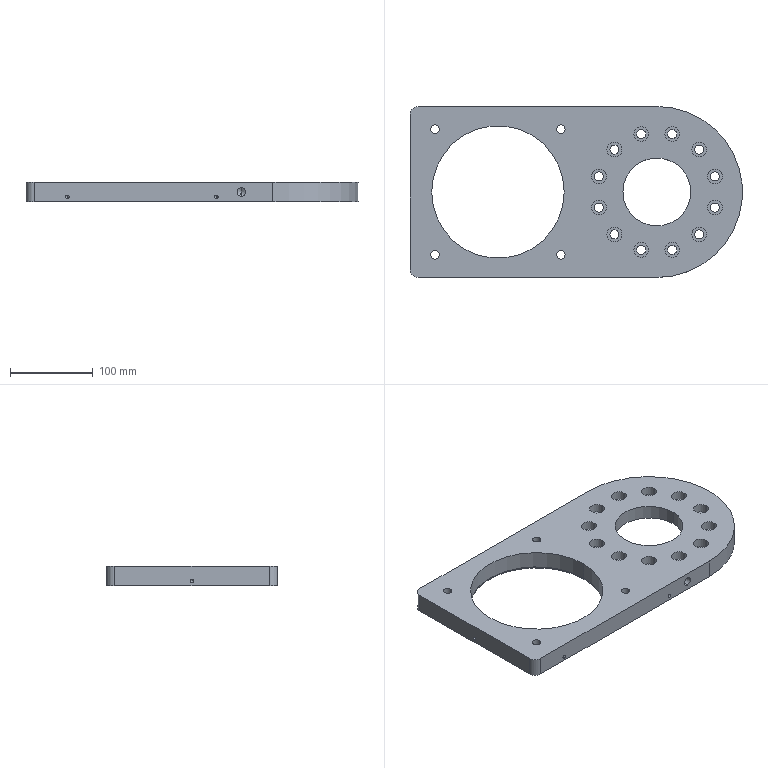Part | SolidWorks | features HoleWzd 6, ICE 3, MirrorPattern 3, Chamfer 2, CirPattern 1, Extrusion 1, Fillet 1 | 1 solid | 115 faces | box 401.6 x 206.6 x 23 mm | volume 1126523 mm3 | cylinder 79 | cone 18 | plane 18 | commonest cylinder face diameters 11 x24 18 x24 10.2 x12 4.2 x10 20 x2 82 x2